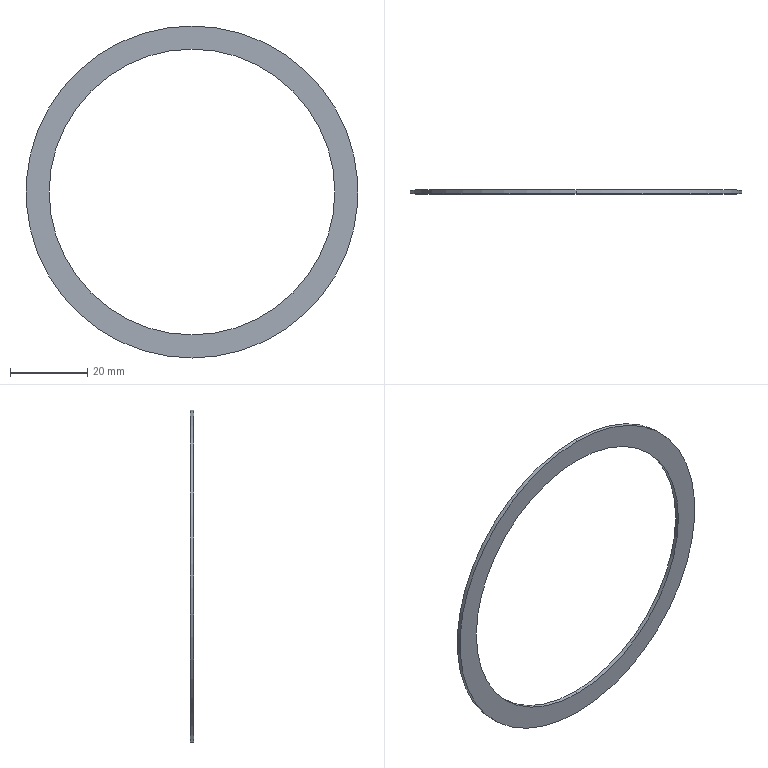Part | SolidWorks | features Extrusion 1 | 1 solid | 6 faces | box 86 x 1 x 86 mm | volume 1508 mm3 | cylinder 4 | plane 2 | commonest cylinder face diameters 74 x2 86 x2
STEP:
#1=CARTESIAN_POINT('',(0.,1.,-37.));
#2=VERTEX_POINT('',#1);
#3=CARTESIAN_POINT('',(0.,1.,37.));
#4=VERTEX_POINT('',#3);
#5=CARTESIAN_POINT('',(0.,1.,0.));
#6=DIRECTION('',(0.,1.,0.));
#7=DIRECTION('',(0.,0.,1.));
#8=AXIS2_PLACEMENT_3D('',#5,#6,#7);
#9=CIRCLE('',#8,37.);
#10=EDGE_CURVE('',#2,#4,#9,.T.);
#11=ORIENTED_EDGE('',*,*,#10,.T.);
#12=CARTESIAN_POINT('',(0.,0.,37.));
#13=VERTEX_POINT('',#12);
#14=CARTESIAN_POINT('',(0.,1.,37.));
#15=DIRECTION('',(0.,-1.,0.));
#16=VECTOR('',#15,1000.);
#17=LINE('',#14,#16);
#18=EDGE_CURVE('',#4,#13,#17,.T.);
#19=ORIENTED_EDGE('',*,*,#18,.T.);
#20=CARTESIAN_POINT('',(0.,0.,-37.));
#21=VERTEX_POINT('',#20);
#22=CARTESIAN_POINT('',(0.,0.,0.));
#23=DIRECTION('',(0.,1.,0.));
#24=DIRECTION('',(0.,0.,1.));
#25=AXIS2_PLACEMENT_3D('',#22,#23,#24);
#26=CIRCLE('',#25,37.);
#27=EDGE_CURVE('',#21,#13,#26,.T.);
#28=ORIENTED_EDGE('',*,*,#27,.F.);
#29=CARTESIAN_POINT('',(0.,1.,-37.));
#30=DIRECTION('',(0.,-1.,0.));
#31=VECTOR('',#30,1000.);
#32=LINE('',#29,#31);
#33=EDGE_CURVE('',#2,#21,#32,.T.);
#34=ORIENTED_EDGE('',*,*,#33,.F.);
#35=EDGE_LOOP('',(#11,#19,#28,#34));
#36=FACE_OUTER_BOUND('',#35,.T.);
#37=CARTESIAN_POINT('',(0.,1.,0.));
#38=DIRECTION('',(0.,-1.,0.));
#39=DIRECTION('',(0.,0.,-1.));
#40=AXIS2_PLACEMENT_3D('',#37,#38,#39);
#41=CYLINDRICAL_SURFACE('',#40,37.);
#42=ADVANCED_FACE('',(#36),#41,.F.);
#43=CARTESIAN_POINT('',(0.,1.,43.));
#44=VERTEX_POINT('',#43);
#45=CARTESIAN_POINT('',(0.,1.,-43.));
#46=VERTEX_POINT('',#45);
#47=CARTESIAN_POINT('',(0.,1.,0.));
#48=DIRECTION('',(0.,1.,0.));
#49=DIRECTION('',(0.,0.,1.));
#50=AXIS2_PLACEMENT_3D('',#47,#48,#49);
#51=CIRCLE('',#50,43.);
#52=EDGE_CURVE('',#44,#46,#51,.T.);
#53=ORIENTED_EDGE('',*,*,#52,.F.);
#54=CARTESIAN_POINT('',(0.,0.,43.));
#55=VERTEX_POINT('',#54);
#56=CARTESIAN_POINT('',(0.,1.,43.));
#57=DIRECTION('',(0.,-1.,0.));
#58=VECTOR('',#57,1000.);
#59=LINE('',#56,#58);
#60=EDGE_CURVE('',#44,#55,#59,.T.);
#61=ORIENTED_EDGE('',*,*,#60,.T.);
#62=CARTESIAN_POINT('',(0.,0.,-43.));
#63=VERTEX_POINT('',#62);
#64=CARTESIAN_POINT('',(0.,0.,0.));
#65=DIRECTION('',(0.,1.,0.));
#66=DIRECTION('',(0.,0.,1.));
#67=AXIS2_PLACEMENT_3D('',#64,#65,#66);
#68=CIRCLE('',#67,43.);
#69=EDGE_CURVE('',#55,#63,#68,.T.);
#70=ORIENTED_EDGE('',*,*,#69,.T.);
#71=CARTESIAN_POINT('',(0.,1.,-43.));
#72=DIRECTION('',(0.,-1.,0.));
#73=VECTOR('',#72,1000.);
#74=LINE('',#71,#73);
#75=EDGE_CURVE('',#46,#63,#74,.T.);
#76=ORIENTED_EDGE('',*,*,#75,.F.);
#77=EDGE_LOOP('',(#53,#61,#70,#76));
#78=FACE_OUTER_BOUND('',#77,.T.);
#79=CARTESIAN_POINT('',(0.,1.,0.));
#80=DIRECTION('',(0.,-1.,0.));
#81=DIRECTION('',(0.,0.,-1.));
#82=AXIS2_PLACEMENT_3D('',#79,#80,#81);
#83=CYLINDRICAL_SURFACE('',#82,43.);
#84=ADVANCED_FACE('',(#78),#83,.T.);
#85=CARTESIAN_POINT('',(0.,1.,0.));
#86=DIRECTION('',(0.,1.,0.));
#87=DIRECTION('',(0.,0.,1.));
#88=AXIS2_PLACEMENT_3D('',#85,#86,#87);
#89=CIRCLE('',#88,43.);
#90=EDGE_CURVE('',#46,#44,#89,.T.);
#91=ORIENTED_EDGE('',*,*,#90,.T.);
#92=ORIENTED_EDGE('',*,*,#52,.T.);
#93=EDGE_LOOP('',(#91,#92));
#94=FACE_OUTER_BOUND('',#93,.T.);
#95=ORIENTED_EDGE('',*,*,#10,.F.);
#96=CARTESIAN_POINT('',(0.,1.,0.));
#97=DIRECTION('',(0.,1.,0.));
#98=DIRECTION('',(0.,0.,1.));
#99=AXIS2_PLACEMENT_3D('',#96,#97,#98);
#100=CIRCLE('',#99,37.);
#101=EDGE_CURVE('',#4,#2,#100,.T.);
#102=ORIENTED_EDGE('',*,*,#101,.F.);
#103=EDGE_LOOP('',(#95,#102));
#104=FACE_BOUND('',#103,.T.);
#105=CARTESIAN_POINT('',(0.,1.,0.));
#106=DIRECTION('',(0.,1.,0.));
#107=DIRECTION('',(0.,0.,1.));
#108=AXIS2_PLACEMENT_3D('',#105,#106,#107);
#109=PLANE('',#108);
#110=ADVANCED_FACE('',(#94,#104),#109,.T.);
#111=CARTESIAN_POINT('',(0.,0.,0.));
#112=DIRECTION('',(0.,1.,0.));
#113=DIRECTION('',(0.,0.,1.));
#114=AXIS2_PLACEMENT_3D('',#111,#112,#113);
#115=CIRCLE('',#114,43.);
#116=EDGE_CURVE('',#63,#55,#115,.T.);
#117=ORIENTED_EDGE('',*,*,#116,.F.);
#118=ORIENTED_EDGE('',*,*,#69,.F.);
#119=EDGE_LOOP('',(#117,#118));
#120=FACE_OUTER_BOUND('',#119,.T.);
#121=ORIENTED_EDGE('',*,*,#27,.T.);
#122=CARTESIAN_POINT('',(0.,0.,0.));
#123=DIRECTION('',(0.,1.,0.));
#124=DIRECTION('',(0.,0.,1.));
#125=AXIS2_PLACEMENT_3D('',#122,#123,#124);
#126=CIRCLE('',#125,37.);
#127=EDGE_CURVE('',#13,#21,#126,.T.);
#128=ORIENTED_EDGE('',*,*,#127,.T.);
#129=EDGE_LOOP('',(#121,#128));
#130=FACE_BOUND('',#129,.T.);
#131=CARTESIAN_POINT('',(0.,0.,0.));
#132=DIRECTION('',(0.,1.,0.));
#133=DIRECTION('',(0.,0.,1.));
#134=AXIS2_PLACEMENT_3D('',#131,#132,#133);
#135=PLANE('',#134);
#136=ADVANCED_FACE('',(#120,#130),#135,.F.);
#137=ORIENTED_EDGE('',*,*,#60,.F.);
#138=ORIENTED_EDGE('',*,*,#90,.F.);
#139=ORIENTED_EDGE('',*,*,#75,.T.);
#140=ORIENTED_EDGE('',*,*,#116,.T.);
#141=EDGE_LOOP('',(#137,#138,#139,#140));
#142=FACE_OUTER_BOUND('',#141,.T.);
#143=CARTESIAN_POINT('',(0.,1.,0.));
#144=DIRECTION('',(0.,-1.,0.));
#145=DIRECTION('',(0.,0.,-1.));
#146=AXIS2_PLACEMENT_3D('',#143,#144,#145);
#147=CYLINDRICAL_SURFACE('',#146,43.);
#148=ADVANCED_FACE('',(#142),#147,.T.);
#149=ORIENTED_EDGE('',*,*,#18,.F.);
#150=ORIENTED_EDGE('',*,*,#101,.T.);
#151=ORIENTED_EDGE('',*,*,#33,.T.);
#152=ORIENTED_EDGE('',*,*,#127,.F.);
#153=EDGE_LOOP('',(#149,#150,#151,#152));
#154=FACE_OUTER_BOUND('',#153,.T.);
#155=CARTESIAN_POINT('',(0.,1.,0.));
#156=DIRECTION('',(0.,-1.,0.));
#157=DIRECTION('',(0.,0.,-1.));
#158=AXIS2_PLACEMENT_3D('',#155,#156,#157);
#159=CYLINDRICAL_SURFACE('',#158,37.);
#160=ADVANCED_FACE('',(#154),#159,.F.);
#161=CLOSED_SHELL('',(#42,#84,#110,#136,#148,#160));
#162=MANIFOLD_SOLID_BREP('',#161);
#163=CARTESIAN_POINT('',(0.,0.,0.));
#164=DIRECTION('',(0.,0.,1.));
#165=DIRECTION('',(1.,0.,0.));
#166=AXIS2_PLACEMENT_3D('',#163,#164,#165);
#167=(LENGTH_UNIT()NAMED_UNIT(*)SI_UNIT(.MILLI.,.METRE.));
#168=UNCERTAINTY_MEASURE_WITH_UNIT(LENGTH_MEASURE(0.00001),#167,'','');
#169=(NAMED_UNIT(*)PLANE_ANGLE_UNIT()SI_UNIT($,.RADIAN.));
#170=(NAMED_UNIT(*)SI_UNIT($,.STERADIAN.)SOLID_ANGLE_UNIT());
#171=(GEOMETRIC_REPRESENTATION_CONTEXT(3)GLOBAL_UNCERTAINTY_ASSIGNED_CONTEXT((#168))GLOBAL_UNIT_ASSIGNED_CONTEXT((#167,#169,#170))REPRESENTATION_CONTEXT('',''));
#172=ADVANCED_BREP_SHAPE_REPRESENTATION('',(#162,#166),#171);